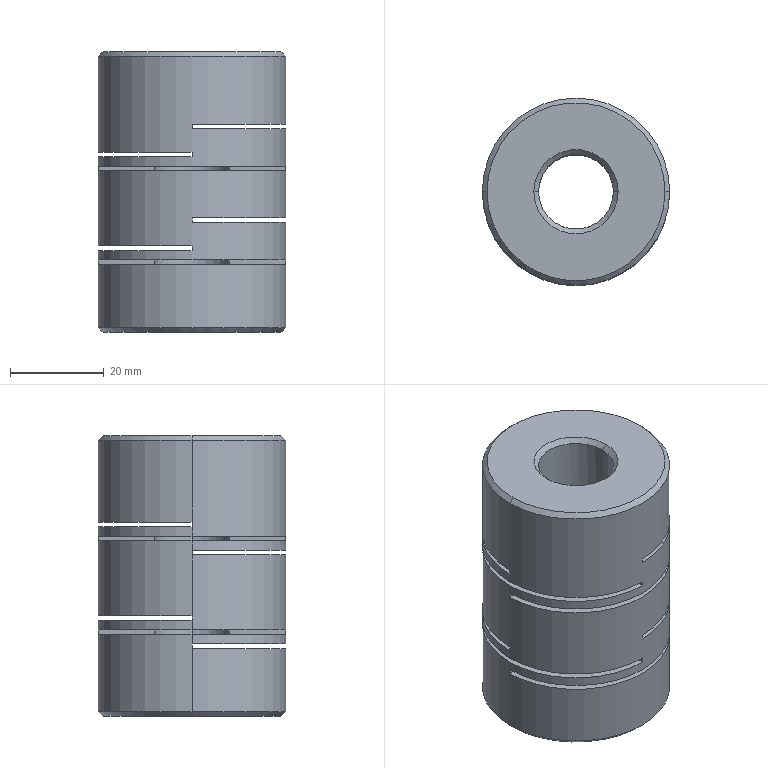Part | STEP file | Coupling | 1 solid | 54 faces | box 40 x 40 x 60 mm | volume 58936 mm3 | plane 34 | cylinder 12 | cone 8 | commonest cylinder face diameters 16 x6 40 x6